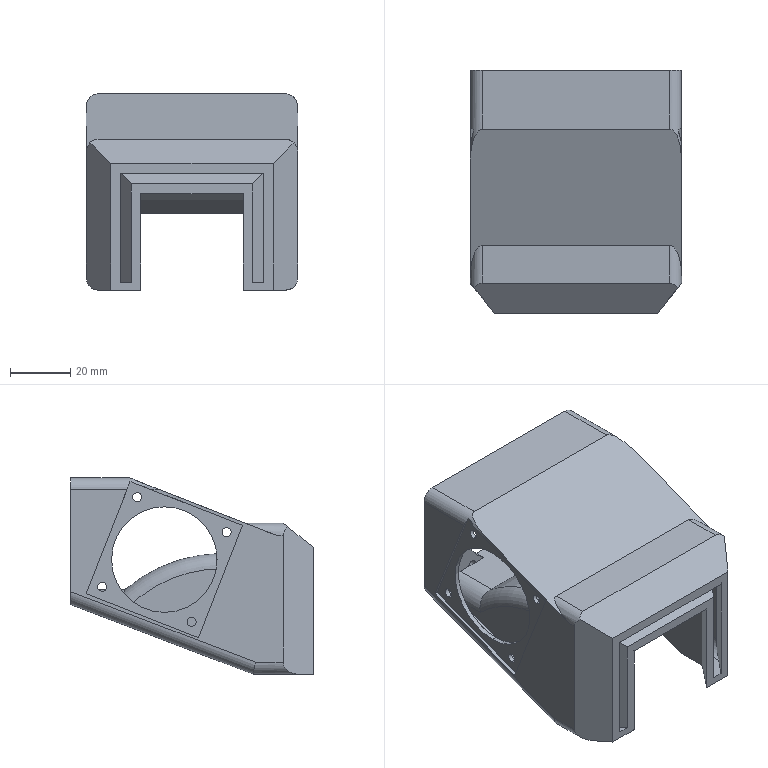Part | STEP file | U-type air nozzle | 1 solid | 132 faces | box 70 x 80.5 x 65.068 mm | volume 54553 mm3 | plane 66 | cylinder 51 | spline 10 | torus 5 | commonest cylinder face diameters 3 x24 8 x13 12 x4 35 x4 1.2 x2 38.164 x2